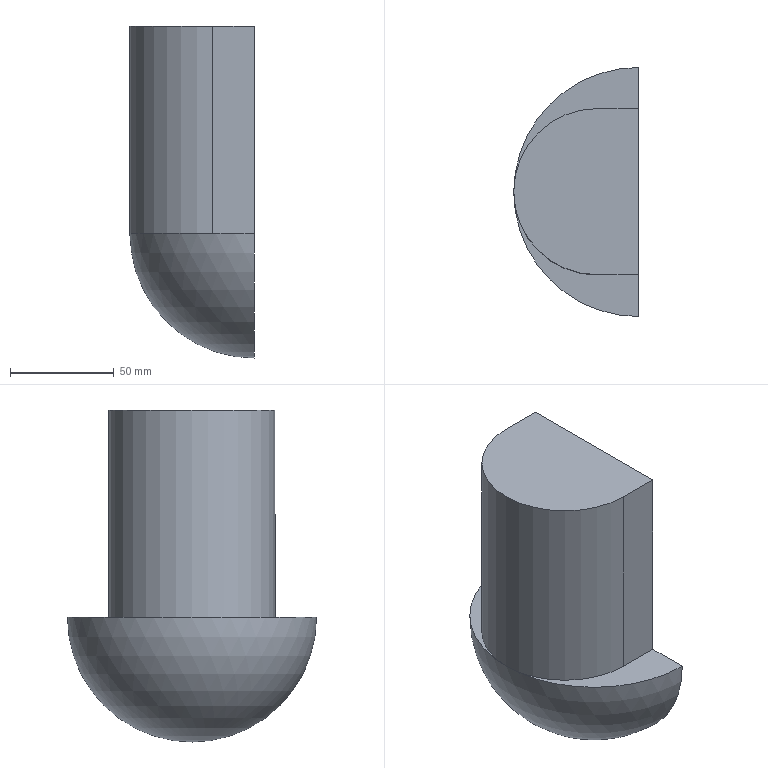Part | SolidWorks | features 3DProfileFeature 1, Extrusion 1, Revolution 1 | 1 solid | 8 faces | box 60 x 120 x 160 mm | volume 637522 mm3 | plane 6 | cylinder 1 | sphere 1 | commonest cylinder face diameters 80 x1
STEP:
#1=CARTESIAN_POINT('',(0.,0.,0.));
#2=VERTEX_POINT('',#1);
#3=CARTESIAN_POINT('',(-20.,0.,0.));
#4=VERTEX_POINT('',#3);
#5=CARTESIAN_POINT('',(-20.,0.,0.));
#6=DIRECTION('',(-1.,0.,0.));
#7=VECTOR('',#6,1000.);
#8=LINE('',#5,#7);
#9=EDGE_CURVE('',#2,#4,#8,.T.);
#10=ORIENTED_EDGE('',*,*,#9,.F.);
#11=CARTESIAN_POINT('',(0.,0.,-100.));
#12=VERTEX_POINT('',#11);
#13=CARTESIAN_POINT('',(0.,0.,-100.));
#14=DIRECTION('',(0.,0.,1.));
#15=VECTOR('',#14,1000.);
#16=LINE('',#13,#15);
#17=EDGE_CURVE('',#12,#2,#16,.T.);
#18=ORIENTED_EDGE('',*,*,#17,.F.);
#19=CARTESIAN_POINT('',(-20.,0.,-100.));
#20=VERTEX_POINT('',#19);
#21=CARTESIAN_POINT('',(-20.,0.,-100.));
#22=DIRECTION('',(-1.,0.,0.));
#23=VECTOR('',#22,1000.);
#24=LINE('',#21,#23);
#25=EDGE_CURVE('',#12,#20,#24,.T.);
#26=ORIENTED_EDGE('',*,*,#25,.T.);
#27=CARTESIAN_POINT('',(-20.,0.,-100.));
#28=DIRECTION('',(0.,0.,1.));
#29=VECTOR('',#28,1000.);
#30=LINE('',#27,#29);
#31=EDGE_CURVE('',#20,#4,#30,.T.);
#32=ORIENTED_EDGE('',*,*,#31,.T.);
#33=EDGE_LOOP('',(#10,#18,#26,#32));
#34=FACE_OUTER_BOUND('',#33,.T.);
#35=CARTESIAN_POINT('',(-20.,0.,-100.));
#36=DIRECTION('',(0.,1.,0.));
#37=DIRECTION('',(0.,0.,1.));
#38=AXIS2_PLACEMENT_3D('',#35,#36,#37);
#39=PLANE('',#38);
#40=ADVANCED_FACE('',(#34),#39,.T.);
#41=CARTESIAN_POINT('',(0.,-80.,0.));
#42=VERTEX_POINT('',#41);
#43=CARTESIAN_POINT('',(0.,0.,0.));
#44=DIRECTION('',(0.,1.,0.));
#45=VECTOR('',#44,1000.);
#46=LINE('',#43,#45);
#47=EDGE_CURVE('',#42,#2,#46,.T.);
#48=ORIENTED_EDGE('',*,*,#47,.F.);
#49=CARTESIAN_POINT('',(0.,-80.,-100.));
#50=VERTEX_POINT('',#49);
#51=CARTESIAN_POINT('',(0.,-80.,-100.));
#52=DIRECTION('',(0.,0.,1.));
#53=VECTOR('',#52,1000.);
#54=LINE('',#51,#53);
#55=EDGE_CURVE('',#50,#42,#54,.T.);
#56=ORIENTED_EDGE('',*,*,#55,.F.);
#57=CARTESIAN_POINT('',(0.,-100.,-100.));
#58=VERTEX_POINT('',#57);
#59=CARTESIAN_POINT('',(0.,20.,-100.));
#60=DIRECTION('',(0.,-1.,0.));
#61=VECTOR('',#60,1000.);
#62=LINE('',#59,#61);
#63=EDGE_CURVE('',#50,#58,#62,.T.);
#64=ORIENTED_EDGE('',*,*,#63,.T.);
#65=CARTESIAN_POINT('',(0.,20.,-100.));
#66=VERTEX_POINT('',#65);
#67=CARTESIAN_POINT('',(0.,-40.,-100.));
#68=DIRECTION('',(1.,0.,0.));
#69=DIRECTION('',(0.,-1.,0.));
#70=AXIS2_PLACEMENT_3D('',#67,#68,#69);
#71=CIRCLE('',#70,60.);
#72=EDGE_CURVE('',#58,#66,#71,.T.);
#73=ORIENTED_EDGE('',*,*,#72,.T.);
#74=CARTESIAN_POINT('',(0.,20.,-100.));
#75=DIRECTION('',(0.,-1.,0.));
#76=VECTOR('',#75,1000.);
#77=LINE('',#74,#76);
#78=EDGE_CURVE('',#66,#12,#77,.T.);
#79=ORIENTED_EDGE('',*,*,#78,.T.);
#80=ORIENTED_EDGE('',*,*,#17,.T.);
#81=EDGE_LOOP('',(#48,#56,#64,#73,#79,#80));
#82=FACE_OUTER_BOUND('',#81,.T.);
#83=CARTESIAN_POINT('',(0.,0.,-100.));
#84=DIRECTION('',(1.,0.,0.));
#85=DIRECTION('',(0.,1.,0.));
#86=AXIS2_PLACEMENT_3D('',#83,#84,#85);
#87=PLANE('',#86);
#88=ADVANCED_FACE('',(#82),#87,.T.);
#89=CARTESIAN_POINT('',(-20.,-80.,0.));
#90=VERTEX_POINT('',#89);
#91=CARTESIAN_POINT('',(0.,-80.,0.));
#92=DIRECTION('',(1.,0.,0.));
#93=VECTOR('',#92,1000.);
#94=LINE('',#91,#93);
#95=EDGE_CURVE('',#90,#42,#94,.T.);
#96=ORIENTED_EDGE('',*,*,#95,.F.);
#97=CARTESIAN_POINT('',(-20.,-80.,-100.));
#98=VERTEX_POINT('',#97);
#99=CARTESIAN_POINT('',(-20.,-80.,-100.));
#100=DIRECTION('',(0.,0.,1.));
#101=VECTOR('',#100,1000.);
#102=LINE('',#99,#101);
#103=EDGE_CURVE('',#98,#90,#102,.T.);
#104=ORIENTED_EDGE('',*,*,#103,.F.);
#105=CARTESIAN_POINT('',(0.,-80.,-100.));
#106=DIRECTION('',(1.,0.,0.));
#107=VECTOR('',#106,1000.);
#108=LINE('',#105,#107);
#109=EDGE_CURVE('',#98,#50,#108,.T.);
#110=ORIENTED_EDGE('',*,*,#109,.T.);
#111=ORIENTED_EDGE('',*,*,#55,.T.);
#112=EDGE_LOOP('',(#96,#104,#110,#111));
#113=FACE_OUTER_BOUND('',#112,.T.);
#114=CARTESIAN_POINT('',(0.,-80.,-100.));
#115=DIRECTION('',(0.,-1.,0.));
#116=DIRECTION('',(0.,0.,-1.));
#117=AXIS2_PLACEMENT_3D('',#114,#115,#116);
#118=PLANE('',#117);
#119=ADVANCED_FACE('',(#113),#118,.T.);
#120=CARTESIAN_POINT('',(-20.,-40.,0.));
#121=DIRECTION('',(0.,0.,1.));
#122=DIRECTION('',(-1.,0.,0.));
#123=AXIS2_PLACEMENT_3D('',#120,#121,#122);
#124=CIRCLE('',#123,40.);
#125=EDGE_CURVE('',#4,#90,#124,.T.);
#126=ORIENTED_EDGE('',*,*,#125,.F.);
#127=ORIENTED_EDGE('',*,*,#31,.F.);
#128=CARTESIAN_POINT('',(-60.,-40.,-100.));
#129=VERTEX_POINT('',#128);
#130=CARTESIAN_POINT('',(-20.,-40.,-100.));
#131=DIRECTION('',(0.,0.,1.));
#132=DIRECTION('',(-1.,0.,0.));
#133=AXIS2_PLACEMENT_3D('',#130,#131,#132);
#134=CIRCLE('',#133,40.);
#135=EDGE_CURVE('',#20,#129,#134,.T.);
#136=ORIENTED_EDGE('',*,*,#135,.T.);
#137=CARTESIAN_POINT('',(-20.,-40.,-100.));
#138=DIRECTION('',(0.,0.,1.));
#139=DIRECTION('',(-1.,0.,0.));
#140=AXIS2_PLACEMENT_3D('',#137,#138,#139);
#141=CIRCLE('',#140,40.);
#142=EDGE_CURVE('',#129,#98,#141,.T.);
#143=ORIENTED_EDGE('',*,*,#142,.T.);
#144=ORIENTED_EDGE('',*,*,#103,.T.);
#145=EDGE_LOOP('',(#126,#127,#136,#143,#144));
#146=FACE_OUTER_BOUND('',#145,.T.);
#147=CARTESIAN_POINT('',(-20.,-40.,-100.));
#148=DIRECTION('',(0.,0.,1.));
#149=DIRECTION('',(1.,0.,0.));
#150=AXIS2_PLACEMENT_3D('',#147,#148,#149);
#151=CYLINDRICAL_SURFACE('',#150,40.);
#152=ADVANCED_FACE('',(#146),#151,.T.);
#153=ORIENTED_EDGE('',*,*,#9,.T.);
#154=ORIENTED_EDGE('',*,*,#125,.T.);
#155=ORIENTED_EDGE('',*,*,#95,.T.);
#156=ORIENTED_EDGE('',*,*,#47,.T.);
#157=EDGE_LOOP('',(#153,#154,#155,#156));
#158=FACE_OUTER_BOUND('',#157,.T.);
#159=CARTESIAN_POINT('',(-20.,-40.,0.));
#160=DIRECTION('',(0.,0.,-1.));
#161=DIRECTION('',(-1.,0.,0.));
#162=AXIS2_PLACEMENT_3D('',#159,#160,#161);
#163=PLANE('',#162);
#164=ADVANCED_FACE('',(#158),#163,.F.);
#165=ORIENTED_EDGE('',*,*,#25,.F.);
#166=ORIENTED_EDGE('',*,*,#78,.F.);
#167=CARTESIAN_POINT('',(0.,-40.,-100.));
#168=DIRECTION('',(0.,0.,-1.));
#169=DIRECTION('',(0.,-1.,0.));
#170=AXIS2_PLACEMENT_3D('',#167,#168,#169);
#171=CIRCLE('',#170,60.);
#172=EDGE_CURVE('',#129,#66,#171,.T.);
#173=ORIENTED_EDGE('',*,*,#172,.F.);
#174=ORIENTED_EDGE('',*,*,#135,.F.);
#175=EDGE_LOOP('',(#165,#166,#173,#174));
#176=FACE_OUTER_BOUND('',#175,.T.);
#177=CARTESIAN_POINT('',(0.,-40.,-100.));
#178=DIRECTION('',(0.,0.,1.));
#179=DIRECTION('',(0.,-1.,0.));
#180=AXIS2_PLACEMENT_3D('',#177,#178,#179);
#181=PLANE('',#180);
#182=ADVANCED_FACE('',(#176),#181,.T.);
#183=ORIENTED_EDGE('',*,*,#109,.F.);
#184=ORIENTED_EDGE('',*,*,#142,.F.);
#185=CARTESIAN_POINT('',(0.,-40.,-100.));
#186=DIRECTION('',(0.,0.,-1.));
#187=DIRECTION('',(0.,-1.,0.));
#188=AXIS2_PLACEMENT_3D('',#185,#186,#187);
#189=CIRCLE('',#188,60.);
#190=EDGE_CURVE('',#58,#129,#189,.T.);
#191=ORIENTED_EDGE('',*,*,#190,.F.);
#192=ORIENTED_EDGE('',*,*,#63,.F.);
#193=EDGE_LOOP('',(#183,#184,#191,#192));
#194=FACE_OUTER_BOUND('',#193,.T.);
#195=CARTESIAN_POINT('',(0.,-40.,-100.));
#196=DIRECTION('',(0.,0.,1.));
#197=DIRECTION('',(0.,-1.,0.));
#198=AXIS2_PLACEMENT_3D('',#195,#196,#197);
#199=PLANE('',#198);
#200=ADVANCED_FACE('',(#194),#199,.T.);
#201=ORIENTED_EDGE('',*,*,#72,.F.);
#202=ORIENTED_EDGE('',*,*,#190,.T.);
#203=ORIENTED_EDGE('',*,*,#172,.T.);
#204=EDGE_LOOP('',(#201,#202,#203));
#205=FACE_OUTER_BOUND('',#204,.T.);
#206=CARTESIAN_POINT('',(0.,-40.,-100.));
#207=DIRECTION('',(0.,0.,1.));
#208=DIRECTION('',(1.,0.,0.));
#209=AXIS2_PLACEMENT_3D('',#206,#207,#208);
#210=SPHERICAL_SURFACE('',#209,60.);
#211=ADVANCED_FACE('',(#205),#210,.T.);
#212=CLOSED_SHELL('',(#40,#88,#119,#152,#164,#182,#200,#211));
#213=MANIFOLD_SOLID_BREP('',#212);
#214=CARTESIAN_POINT('',(0.,0.,0.));
#215=DIRECTION('',(0.,0.,1.));
#216=DIRECTION('',(1.,0.,0.));
#217=AXIS2_PLACEMENT_3D('',#214,#215,#216);
#218=(LENGTH_UNIT()NAMED_UNIT(*)SI_UNIT(.MILLI.,.METRE.));
#219=UNCERTAINTY_MEASURE_WITH_UNIT(LENGTH_MEASURE(0.00001),#218,'','');
#220=(NAMED_UNIT(*)PLANE_ANGLE_UNIT()SI_UNIT($,.RADIAN.));
#221=(NAMED_UNIT(*)SI_UNIT($,.STERADIAN.)SOLID_ANGLE_UNIT());
#222=(GEOMETRIC_REPRESENTATION_CONTEXT(3)GLOBAL_UNCERTAINTY_ASSIGNED_CONTEXT((#219))GLOBAL_UNIT_ASSIGNED_CONTEXT((#218,#220,#221))REPRESENTATION_CONTEXT('',''));
#223=ADVANCED_BREP_SHAPE_REPRESENTATION('',(#213,#217),#222);